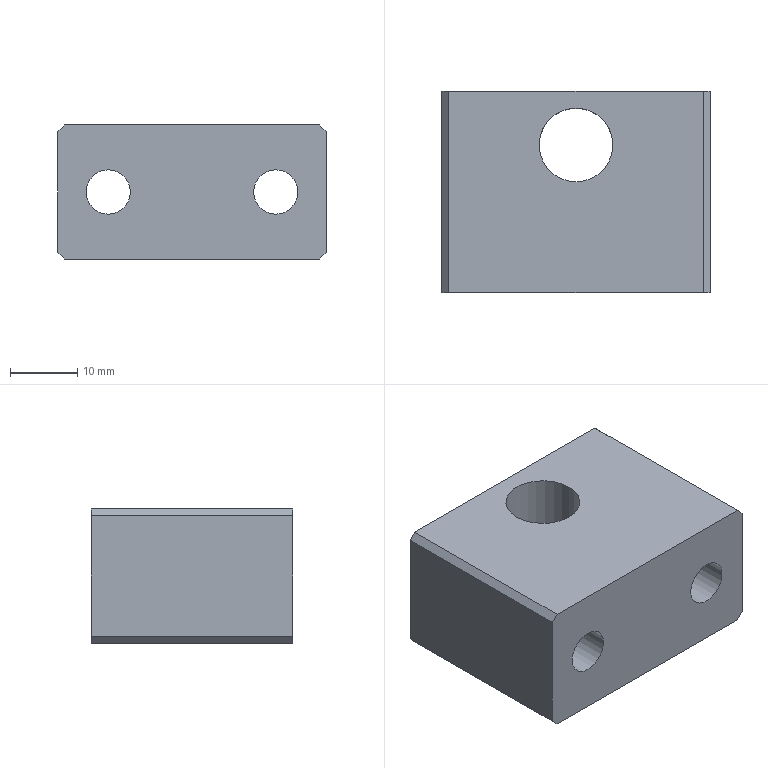Part | NX | 1 solid | 17 faces | box 40 x 30 x 20 mm | volume 19208 mm3 | plane 12 | cylinder 5 | commonest cylinder face diameters 11 x3 6.6 x2
STEP:
#1=CARTESIAN_POINT('',(20.,0.,9.));
#2=VERTEX_POINT('',#1);
#3=CARTESIAN_POINT('',(20.,0.,-9.));
#4=VERTEX_POINT('',#3);
#5=CARTESIAN_POINT('',(20.,0.,10.));
#6=DIRECTION('',(0.,0.,-1.));
#7=VECTOR('',#6,1000.);
#8=LINE('',#5,#7);
#9=EDGE_CURVE('',#2,#4,#8,.T.);
#10=ORIENTED_EDGE('',*,*,#9,.T.);
#11=CARTESIAN_POINT('',(20.,30.,-9.));
#12=VERTEX_POINT('',#11);
#13=CARTESIAN_POINT('',(20.,30.,-9.));
#14=DIRECTION('',(0.,1.,0.));
#15=VECTOR('',#14,1000.);
#16=LINE('',#13,#15);
#17=EDGE_CURVE('',#4,#12,#16,.T.);
#18=ORIENTED_EDGE('',*,*,#17,.T.);
#19=CARTESIAN_POINT('',(20.,30.,9.));
#20=VERTEX_POINT('',#19);
#21=CARTESIAN_POINT('',(20.,30.,10.));
#22=DIRECTION('',(0.,0.,-1.));
#23=VECTOR('',#22,1000.);
#24=LINE('',#21,#23);
#25=EDGE_CURVE('',#20,#12,#24,.T.);
#26=ORIENTED_EDGE('',*,*,#25,.F.);
#27=CARTESIAN_POINT('',(20.,30.,9.));
#28=DIRECTION('',(0.,-1.,0.));
#29=VECTOR('',#28,1000.);
#30=LINE('',#27,#29);
#31=EDGE_CURVE('',#20,#2,#30,.T.);
#32=ORIENTED_EDGE('',*,*,#31,.T.);
#33=EDGE_LOOP('',(#10,#18,#26,#32));
#34=FACE_BOUND('',#33,.T.);
#35=CARTESIAN_POINT('',(20.,30.,10.));
#36=DIRECTION('',(-1.,0.,0.));
#37=DIRECTION('',(0.,0.,1.));
#38=AXIS2_PLACEMENT_3D('',#35,#36,#37);
#39=PLANE('',#38);
#40=ADVANCED_FACE('',(#34),#39,.F.);
#41=CARTESIAN_POINT('',(5.5,22.,-10.));
#42=VERTEX_POINT('',#41);
#43=CARTESIAN_POINT('',(0.,22.,-10.));
#44=DIRECTION('',(0.,0.,1.));
#45=DIRECTION('',(1.,0.,0.));
#46=AXIS2_PLACEMENT_3D('',#43,#44,#45);
#47=CIRCLE('',#46,5.5);
#48=EDGE_CURVE('',#42,#42,#47,.T.);
#49=ORIENTED_EDGE('',*,*,#48,.T.);
#50=EDGE_LOOP('',(#49));
#51=FACE_BOUND('',#50,.T.);
#52=CARTESIAN_POINT('',(19.,0.,-10.));
#53=VERTEX_POINT('',#52);
#54=CARTESIAN_POINT('',(-19.,0.,-10.));
#55=VERTEX_POINT('',#54);
#56=CARTESIAN_POINT('',(-20.,0.,-10.));
#57=DIRECTION('',(-1.,0.,0.));
#58=VECTOR('',#57,1000.);
#59=LINE('',#56,#58);
#60=EDGE_CURVE('',#53,#55,#59,.T.);
#61=ORIENTED_EDGE('',*,*,#60,.T.);
#62=CARTESIAN_POINT('',(-19.,30.,-10.));
#63=VERTEX_POINT('',#62);
#64=CARTESIAN_POINT('',(-19.,30.,-10.));
#65=DIRECTION('',(0.,1.,0.));
#66=VECTOR('',#65,1000.);
#67=LINE('',#64,#66);
#68=EDGE_CURVE('',#55,#63,#67,.T.);
#69=ORIENTED_EDGE('',*,*,#68,.T.);
#70=CARTESIAN_POINT('',(19.,30.,-10.));
#71=VERTEX_POINT('',#70);
#72=CARTESIAN_POINT('',(-20.,30.,-10.));
#73=DIRECTION('',(-1.,0.,0.));
#74=VECTOR('',#73,1000.);
#75=LINE('',#72,#74);
#76=EDGE_CURVE('',#71,#63,#75,.T.);
#77=ORIENTED_EDGE('',*,*,#76,.F.);
#78=CARTESIAN_POINT('',(19.,30.,-10.));
#79=DIRECTION('',(0.,-1.,0.));
#80=VECTOR('',#79,1000.);
#81=LINE('',#78,#80);
#82=EDGE_CURVE('',#71,#53,#81,.T.);
#83=ORIENTED_EDGE('',*,*,#82,.T.);
#84=EDGE_LOOP('',(#61,#69,#77,#83));
#85=FACE_BOUND('',#84,.T.);
#86=CARTESIAN_POINT('',(-20.,30.,-10.));
#87=DIRECTION('',(0.,0.,1.));
#88=DIRECTION('',(1.,0.,0.));
#89=AXIS2_PLACEMENT_3D('',#86,#87,#88);
#90=PLANE('',#89);
#91=ADVANCED_FACE('',(#51,#85),#90,.F.);
#92=CARTESIAN_POINT('',(-20.,30.,-9.));
#93=VERTEX_POINT('',#92);
#94=CARTESIAN_POINT('',(-20.,30.,9.));
#95=VERTEX_POINT('',#94);
#96=CARTESIAN_POINT('',(-20.,30.,10.));
#97=DIRECTION('',(0.,0.,1.));
#98=VECTOR('',#97,1000.);
#99=LINE('',#96,#98);
#100=EDGE_CURVE('',#93,#95,#99,.T.);
#101=ORIENTED_EDGE('',*,*,#100,.F.);
#102=CARTESIAN_POINT('',(-20.,0.,-9.));
#103=VERTEX_POINT('',#102);
#104=CARTESIAN_POINT('',(-20.,30.,-9.));
#105=DIRECTION('',(0.,-1.,0.));
#106=VECTOR('',#105,1000.);
#107=LINE('',#104,#106);
#108=EDGE_CURVE('',#93,#103,#107,.T.);
#109=ORIENTED_EDGE('',*,*,#108,.T.);
#110=CARTESIAN_POINT('',(-20.,0.,9.));
#111=VERTEX_POINT('',#110);
#112=CARTESIAN_POINT('',(-20.,0.,10.));
#113=DIRECTION('',(0.,0.,1.));
#114=VECTOR('',#113,1000.);
#115=LINE('',#112,#114);
#116=EDGE_CURVE('',#103,#111,#115,.T.);
#117=ORIENTED_EDGE('',*,*,#116,.T.);
#118=CARTESIAN_POINT('',(-20.,30.,9.));
#119=DIRECTION('',(0.,1.,0.));
#120=VECTOR('',#119,1000.);
#121=LINE('',#118,#120);
#122=EDGE_CURVE('',#111,#95,#121,.T.);
#123=ORIENTED_EDGE('',*,*,#122,.T.);
#124=EDGE_LOOP('',(#101,#109,#117,#123));
#125=FACE_BOUND('',#124,.T.);
#126=CARTESIAN_POINT('',(-20.,30.,10.));
#127=DIRECTION('',(1.,0.,0.));
#128=DIRECTION('',(0.,0.,-1.));
#129=AXIS2_PLACEMENT_3D('',#126,#127,#128);
#130=PLANE('',#129);
#131=ADVANCED_FACE('',(#125),#130,.F.);
#132=CARTESIAN_POINT('',(5.5,22.,10.));
#133=VERTEX_POINT('',#132);
#134=CARTESIAN_POINT('',(0.,22.,10.));
#135=DIRECTION('',(0.,0.,1.));
#136=DIRECTION('',(1.,0.,0.));
#137=AXIS2_PLACEMENT_3D('',#134,#135,#136);
#138=CIRCLE('',#137,5.5);
#139=EDGE_CURVE('',#133,#133,#138,.T.);
#140=ORIENTED_EDGE('',*,*,#139,.F.);
#141=EDGE_LOOP('',(#140));
#142=FACE_BOUND('',#141,.T.);
#143=CARTESIAN_POINT('',(-19.,0.,10.));
#144=VERTEX_POINT('',#143);
#145=CARTESIAN_POINT('',(19.,0.,10.));
#146=VERTEX_POINT('',#145);
#147=CARTESIAN_POINT('',(-20.,0.,10.));
#148=DIRECTION('',(1.,0.,0.));
#149=VECTOR('',#148,1000.);
#150=LINE('',#147,#149);
#151=EDGE_CURVE('',#144,#146,#150,.T.);
#152=ORIENTED_EDGE('',*,*,#151,.T.);
#153=CARTESIAN_POINT('',(19.,30.,10.));
#154=VERTEX_POINT('',#153);
#155=CARTESIAN_POINT('',(19.,30.,10.));
#156=DIRECTION('',(0.,1.,0.));
#157=VECTOR('',#156,1000.);
#158=LINE('',#155,#157);
#159=EDGE_CURVE('',#146,#154,#158,.T.);
#160=ORIENTED_EDGE('',*,*,#159,.T.);
#161=CARTESIAN_POINT('',(-19.,30.,10.));
#162=VERTEX_POINT('',#161);
#163=CARTESIAN_POINT('',(-20.,30.,10.));
#164=DIRECTION('',(1.,0.,0.));
#165=VECTOR('',#164,1000.);
#166=LINE('',#163,#165);
#167=EDGE_CURVE('',#162,#154,#166,.T.);
#168=ORIENTED_EDGE('',*,*,#167,.F.);
#169=CARTESIAN_POINT('',(-19.,30.,10.));
#170=DIRECTION('',(0.,-1.,0.));
#171=VECTOR('',#170,1000.);
#172=LINE('',#169,#171);
#173=EDGE_CURVE('',#162,#144,#172,.T.);
#174=ORIENTED_EDGE('',*,*,#173,.T.);
#175=EDGE_LOOP('',(#152,#160,#168,#174));
#176=FACE_BOUND('',#175,.T.);
#177=CARTESIAN_POINT('',(-20.,30.,10.));
#178=DIRECTION('',(0.,0.,-1.));
#179=DIRECTION('',(-1.,0.,0.));
#180=AXIS2_PLACEMENT_3D('',#177,#178,#179);
#181=PLANE('',#180);
#182=ADVANCED_FACE('',(#142,#176),#181,.F.);
#183=CARTESIAN_POINT('',(-12.5,30.,5.5));
#184=VERTEX_POINT('',#183);
#185=CARTESIAN_POINT('',(-12.5,30.,0.));
#186=DIRECTION('',(0.,1.,0.));
#187=DIRECTION('',(0.,0.,1.));
#188=AXIS2_PLACEMENT_3D('',#185,#186,#187);
#189=CIRCLE('',#188,5.5);
#190=EDGE_CURVE('',#184,#184,#189,.T.);
#191=ORIENTED_EDGE('',*,*,#190,.F.);
#192=EDGE_LOOP('',(#191));
#193=FACE_BOUND('',#192,.T.);
#194=CARTESIAN_POINT('',(12.5,30.,5.5));
#195=VERTEX_POINT('',#194);
#196=CARTESIAN_POINT('',(12.5,30.,0.));
#197=DIRECTION('',(0.,1.,0.));
#198=DIRECTION('',(0.,0.,1.));
#199=AXIS2_PLACEMENT_3D('',#196,#197,#198);
#200=CIRCLE('',#199,5.5);
#201=EDGE_CURVE('',#195,#195,#200,.T.);
#202=ORIENTED_EDGE('',*,*,#201,.F.);
#203=EDGE_LOOP('',(#202));
#204=FACE_BOUND('',#203,.T.);
#205=ORIENTED_EDGE('',*,*,#76,.T.);
#206=CARTESIAN_POINT('',(-20.,30.,-9.));
#207=DIRECTION('',(0.7071,0.,-0.7071));
#208=VECTOR('',#207,1000.);
#209=LINE('',#206,#208);
#210=EDGE_CURVE('',#63,#93,#209,.F.);
#211=ORIENTED_EDGE('',*,*,#210,.T.);
#212=ORIENTED_EDGE('',*,*,#100,.T.);
#213=CARTESIAN_POINT('',(-19.,30.,10.));
#214=DIRECTION('',(-0.7071,0.,-0.7071));
#215=VECTOR('',#214,1000.);
#216=LINE('',#213,#215);
#217=EDGE_CURVE('',#95,#162,#216,.F.);
#218=ORIENTED_EDGE('',*,*,#217,.T.);
#219=ORIENTED_EDGE('',*,*,#167,.T.);
#220=CARTESIAN_POINT('',(20.,30.,9.));
#221=DIRECTION('',(-0.7071,0.,0.7071));
#222=VECTOR('',#221,1000.);
#223=LINE('',#220,#222);
#224=EDGE_CURVE('',#154,#20,#223,.F.);
#225=ORIENTED_EDGE('',*,*,#224,.T.);
#226=ORIENTED_EDGE('',*,*,#25,.T.);
#227=CARTESIAN_POINT('',(19.,30.,-10.));
#228=DIRECTION('',(0.7071,0.,0.7071));
#229=VECTOR('',#228,1000.);
#230=LINE('',#227,#229);
#231=EDGE_CURVE('',#12,#71,#230,.F.);
#232=ORIENTED_EDGE('',*,*,#231,.T.);
#233=EDGE_LOOP('',(#205,#211,#212,#218,#219,#225,#226,#232));
#234=FACE_BOUND('',#233,.T.);
#235=CARTESIAN_POINT('',(0.,30.,0.));
#236=DIRECTION('',(0.,-1.,0.));
#237=DIRECTION('',(0.,0.,-1.));
#238=AXIS2_PLACEMENT_3D('',#235,#236,#237);
#239=PLANE('',#238);
#240=ADVANCED_FACE('',(#193,#204,#234),#239,.F.);
#241=CARTESIAN_POINT('',(-12.5,0.,3.3));
#242=VERTEX_POINT('',#241);
#243=CARTESIAN_POINT('',(-12.5,0.,0.));
#244=DIRECTION('',(0.,1.,0.));
#245=DIRECTION('',(0.,0.,1.));
#246=AXIS2_PLACEMENT_3D('',#243,#244,#245);
#247=CIRCLE('',#246,3.3);
#248=EDGE_CURVE('',#242,#242,#247,.T.);
#249=ORIENTED_EDGE('',*,*,#248,.T.);
#250=EDGE_LOOP('',(#249));
#251=FACE_BOUND('',#250,.T.);
#252=CARTESIAN_POINT('',(12.5,0.,3.3));
#253=VERTEX_POINT('',#252);
#254=CARTESIAN_POINT('',(12.5,0.,0.));
#255=DIRECTION('',(0.,1.,0.));
#256=DIRECTION('',(0.,0.,1.));
#257=AXIS2_PLACEMENT_3D('',#254,#255,#256);
#258=CIRCLE('',#257,3.3);
#259=EDGE_CURVE('',#253,#253,#258,.T.);
#260=ORIENTED_EDGE('',*,*,#259,.T.);
#261=EDGE_LOOP('',(#260));
#262=FACE_BOUND('',#261,.T.);
#263=ORIENTED_EDGE('',*,*,#116,.F.);
#264=CARTESIAN_POINT('',(-14.5,0.,-14.5));
#265=DIRECTION('',(-0.7071,0.,0.7071));
#266=VECTOR('',#265,1000.);
#267=LINE('',#264,#266);
#268=EDGE_CURVE('',#103,#55,#267,.F.);
#269=ORIENTED_EDGE('',*,*,#268,.T.);
#270=ORIENTED_EDGE('',*,*,#60,.F.);
#271=CARTESIAN_POINT('',(14.5,0.,-14.5));
#272=DIRECTION('',(-0.7071,0.,-0.7071));
#273=VECTOR('',#272,1000.);
#274=LINE('',#271,#273);
#275=EDGE_CURVE('',#53,#4,#274,.F.);
#276=ORIENTED_EDGE('',*,*,#275,.T.);
#277=ORIENTED_EDGE('',*,*,#9,.F.);
#278=CARTESIAN_POINT('',(14.5,0.,14.5));
#279=DIRECTION('',(0.7071,0.,-0.7071));
#280=VECTOR('',#279,1000.);
#281=LINE('',#278,#280);
#282=EDGE_CURVE('',#2,#146,#281,.F.);
#283=ORIENTED_EDGE('',*,*,#282,.T.);
#284=ORIENTED_EDGE('',*,*,#151,.F.);
#285=CARTESIAN_POINT('',(-14.5,0.,14.5));
#286=DIRECTION('',(0.7071,0.,0.7071));
#287=VECTOR('',#286,1000.);
#288=LINE('',#285,#287);
#289=EDGE_CURVE('',#144,#111,#288,.F.);
#290=ORIENTED_EDGE('',*,*,#289,.T.);
#291=EDGE_LOOP('',(#263,#269,#270,#276,#277,#283,#284,#290));
#292=FACE_BOUND('',#291,.T.);
#293=CARTESIAN_POINT('',(0.,0.,0.));
#294=DIRECTION('',(0.,-1.,0.));
#295=DIRECTION('',(0.,0.,-1.));
#296=AXIS2_PLACEMENT_3D('',#293,#294,#295);
#297=PLANE('',#296);
#298=ADVANCED_FACE('',(#251,#262,#292),#297,.T.);
#299=ORIENTED_EDGE('',*,*,#259,.F.);
#300=EDGE_LOOP('',(#299));
#301=FACE_BOUND('',#300,.T.);
#302=CARTESIAN_POINT('',(12.5,23.6,3.3));
#303=VERTEX_POINT('',#302);
#304=CARTESIAN_POINT('',(12.5,23.6,0.));
#305=DIRECTION('',(0.,1.,0.));
#306=DIRECTION('',(0.,0.,1.));
#307=AXIS2_PLACEMENT_3D('',#304,#305,#306);
#308=CIRCLE('',#307,3.3);
#309=EDGE_CURVE('',#303,#303,#308,.T.);
#310=ORIENTED_EDGE('',*,*,#309,.T.);
#311=EDGE_LOOP('',(#310));
#312=FACE_BOUND('',#311,.T.);
#313=CARTESIAN_POINT('',(12.5,30.,0.));
#314=DIRECTION('',(0.,1.,0.));
#315=DIRECTION('',(0.,0.,1.));
#316=AXIS2_PLACEMENT_3D('',#313,#314,#315);
#317=CYLINDRICAL_SURFACE('',#316,3.3);
#318=ADVANCED_FACE('',(#301,#312),#317,.F.);
#319=ORIENTED_EDGE('',*,*,#309,.F.);
#320=EDGE_LOOP('',(#319));
#321=FACE_BOUND('',#320,.T.);
#322=CARTESIAN_POINT('',(12.5,23.6,5.5));
#323=VERTEX_POINT('',#322);
#324=CARTESIAN_POINT('',(12.5,23.6,0.));
#325=DIRECTION('',(0.,1.,0.));
#326=DIRECTION('',(0.,0.,1.));
#327=AXIS2_PLACEMENT_3D('',#324,#325,#326);
#328=CIRCLE('',#327,5.5);
#329=EDGE_CURVE('',#323,#323,#328,.T.);
#330=ORIENTED_EDGE('',*,*,#329,.T.);
#331=EDGE_LOOP('',(#330));
#332=FACE_BOUND('',#331,.T.);
#333=CARTESIAN_POINT('',(15.8,23.6,0.));
#334=DIRECTION('',(0.,-1.,0.));
#335=DIRECTION('',(0.,0.,-1.));
#336=AXIS2_PLACEMENT_3D('',#333,#334,#335);
#337=PLANE('',#336);
#338=ADVANCED_FACE('',(#321,#332),#337,.F.);
#339=ORIENTED_EDGE('',*,*,#329,.F.);
#340=EDGE_LOOP('',(#339));
#341=FACE_BOUND('',#340,.T.);
#342=ORIENTED_EDGE('',*,*,#201,.T.);
#343=EDGE_LOOP('',(#342));
#344=FACE_BOUND('',#343,.T.);
#345=CARTESIAN_POINT('',(12.5,30.,0.));
#346=DIRECTION('',(0.,1.,0.));
#347=DIRECTION('',(0.,0.,1.));
#348=AXIS2_PLACEMENT_3D('',#345,#346,#347);
#349=CYLINDRICAL_SURFACE('',#348,5.5);
#350=ADVANCED_FACE('',(#341,#344),#349,.F.);
#351=ORIENTED_EDGE('',*,*,#248,.F.);
#352=EDGE_LOOP('',(#351));
#353=FACE_BOUND('',#352,.T.);
#354=CARTESIAN_POINT('',(-12.5,23.6,3.3));
#355=VERTEX_POINT('',#354);
#356=CARTESIAN_POINT('',(-12.5,23.6,0.));
#357=DIRECTION('',(0.,1.,0.));
#358=DIRECTION('',(0.,0.,1.));
#359=AXIS2_PLACEMENT_3D('',#356,#357,#358);
#360=CIRCLE('',#359,3.3);
#361=EDGE_CURVE('',#355,#355,#360,.T.);
#362=ORIENTED_EDGE('',*,*,#361,.T.);
#363=EDGE_LOOP('',(#362));
#364=FACE_BOUND('',#363,.T.);
#365=CARTESIAN_POINT('',(-12.5,30.,0.));
#366=DIRECTION('',(0.,1.,0.));
#367=DIRECTION('',(0.,0.,1.));
#368=AXIS2_PLACEMENT_3D('',#365,#366,#367);
#369=CYLINDRICAL_SURFACE('',#368,3.3);
#370=ADVANCED_FACE('',(#353,#364),#369,.F.);
#371=ORIENTED_EDGE('',*,*,#361,.F.);
#372=EDGE_LOOP('',(#371));
#373=FACE_BOUND('',#372,.T.);
#374=CARTESIAN_POINT('',(-12.5,23.6,5.5));
#375=VERTEX_POINT('',#374);
#376=CARTESIAN_POINT('',(-12.5,23.6,0.));
#377=DIRECTION('',(0.,1.,0.));
#378=DIRECTION('',(0.,0.,1.));
#379=AXIS2_PLACEMENT_3D('',#376,#377,#378);
#380=CIRCLE('',#379,5.5);
#381=EDGE_CURVE('',#375,#375,#380,.T.);
#382=ORIENTED_EDGE('',*,*,#381,.T.);
#383=EDGE_LOOP('',(#382));
#384=FACE_BOUND('',#383,.T.);
#385=CARTESIAN_POINT('',(-9.2,23.6,0.));
#386=DIRECTION('',(0.,-1.,0.));
#387=DIRECTION('',(0.,0.,-1.));
#388=AXIS2_PLACEMENT_3D('',#385,#386,#387);
#389=PLANE('',#388);
#390=ADVANCED_FACE('',(#373,#384),#389,.F.);
#391=ORIENTED_EDGE('',*,*,#381,.F.);
#392=EDGE_LOOP('',(#391));
#393=FACE_BOUND('',#392,.T.);
#394=ORIENTED_EDGE('',*,*,#190,.T.);
#395=EDGE_LOOP('',(#394));
#396=FACE_BOUND('',#395,.T.);
#397=CARTESIAN_POINT('',(-12.5,30.,0.));
#398=DIRECTION('',(0.,1.,0.));
#399=DIRECTION('',(0.,0.,1.));
#400=AXIS2_PLACEMENT_3D('',#397,#398,#399);
#401=CYLINDRICAL_SURFACE('',#400,5.5);
#402=ADVANCED_FACE('',(#393,#396),#401,.F.);
#403=ORIENTED_EDGE('',*,*,#48,.F.);
#404=EDGE_LOOP('',(#403));
#405=FACE_BOUND('',#404,.T.);
#406=ORIENTED_EDGE('',*,*,#139,.T.);
#407=EDGE_LOOP('',(#406));
#408=FACE_BOUND('',#407,.T.);
#409=CARTESIAN_POINT('',(0.,22.,10.));
#410=DIRECTION('',(0.,0.,1.));
#411=DIRECTION('',(1.,0.,0.));
#412=AXIS2_PLACEMENT_3D('',#409,#410,#411);
#413=CYLINDRICAL_SURFACE('',#412,5.5);
#414=ADVANCED_FACE('',(#405,#408),#413,.F.);
#415=ORIENTED_EDGE('',*,*,#210,.F.);
#416=ORIENTED_EDGE('',*,*,#68,.F.);
#417=ORIENTED_EDGE('',*,*,#268,.F.);
#418=ORIENTED_EDGE('',*,*,#108,.F.);
#419=EDGE_LOOP('',(#415,#416,#417,#418));
#420=FACE_BOUND('',#419,.T.);
#421=CARTESIAN_POINT('',(-20.,30.,-9.));
#422=DIRECTION('',(0.7071,0.,0.7071));
#423=DIRECTION('',(0.,-1.,0.));
#424=AXIS2_PLACEMENT_3D('',#421,#422,#423);
#425=PLANE('',#424);
#426=ADVANCED_FACE('',(#420),#425,.F.);
#427=ORIENTED_EDGE('',*,*,#231,.F.);
#428=ORIENTED_EDGE('',*,*,#17,.F.);
#429=ORIENTED_EDGE('',*,*,#275,.F.);
#430=ORIENTED_EDGE('',*,*,#82,.F.);
#431=EDGE_LOOP('',(#427,#428,#429,#430));
#432=FACE_BOUND('',#431,.T.);
#433=CARTESIAN_POINT('',(19.,30.,-10.));
#434=DIRECTION('',(-0.7071,0.,0.7071));
#435=DIRECTION('',(0.,-1.,0.));
#436=AXIS2_PLACEMENT_3D('',#433,#434,#435);
#437=PLANE('',#436);
#438=ADVANCED_FACE('',(#432),#437,.F.);
#439=ORIENTED_EDGE('',*,*,#224,.F.);
#440=ORIENTED_EDGE('',*,*,#159,.F.);
#441=ORIENTED_EDGE('',*,*,#282,.F.);
#442=ORIENTED_EDGE('',*,*,#31,.F.);
#443=EDGE_LOOP('',(#439,#440,#441,#442));
#444=FACE_BOUND('',#443,.T.);
#445=CARTESIAN_POINT('',(20.,30.,9.));
#446=DIRECTION('',(-0.7071,0.,-0.7071));
#447=DIRECTION('',(0.,-1.,0.));
#448=AXIS2_PLACEMENT_3D('',#445,#446,#447);
#449=PLANE('',#448);
#450=ADVANCED_FACE('',(#444),#449,.F.);
#451=ORIENTED_EDGE('',*,*,#217,.F.);
#452=ORIENTED_EDGE('',*,*,#122,.F.);
#453=ORIENTED_EDGE('',*,*,#289,.F.);
#454=ORIENTED_EDGE('',*,*,#173,.F.);
#455=EDGE_LOOP('',(#451,#452,#453,#454));
#456=FACE_BOUND('',#455,.T.);
#457=CARTESIAN_POINT('',(-19.,30.,10.));
#458=DIRECTION('',(0.7071,0.,-0.7071));
#459=DIRECTION('',(0.,-1.,0.));
#460=AXIS2_PLACEMENT_3D('',#457,#458,#459);
#461=PLANE('',#460);
#462=ADVANCED_FACE('',(#456),#461,.F.);
#463=CLOSED_SHELL('',(#40,#91,#131,#182,#240,#298,#318,#338,#350,#370,#390,#402,#414,#426,#438,#450,#462));
#464=MANIFOLD_SOLID_BREP('',#463);
#465=(LENGTH_UNIT()NAMED_UNIT(*)SI_UNIT(.MILLI.,.METRE.));
#466=UNCERTAINTY_MEASURE_WITH_UNIT(LENGTH_MEASURE(0.00001),#465,'','');
#467=(NAMED_UNIT(*)PLANE_ANGLE_UNIT()SI_UNIT($,.RADIAN.));
#468=(NAMED_UNIT(*)SI_UNIT($,.STERADIAN.)SOLID_ANGLE_UNIT());
#469=(GEOMETRIC_REPRESENTATION_CONTEXT(3)GLOBAL_UNCERTAINTY_ASSIGNED_CONTEXT((#466))GLOBAL_UNIT_ASSIGNED_CONTEXT((#465,#467,#468))REPRESENTATION_CONTEXT('',''));
#470=ADVANCED_BREP_SHAPE_REPRESENTATION('',(#464),#469);